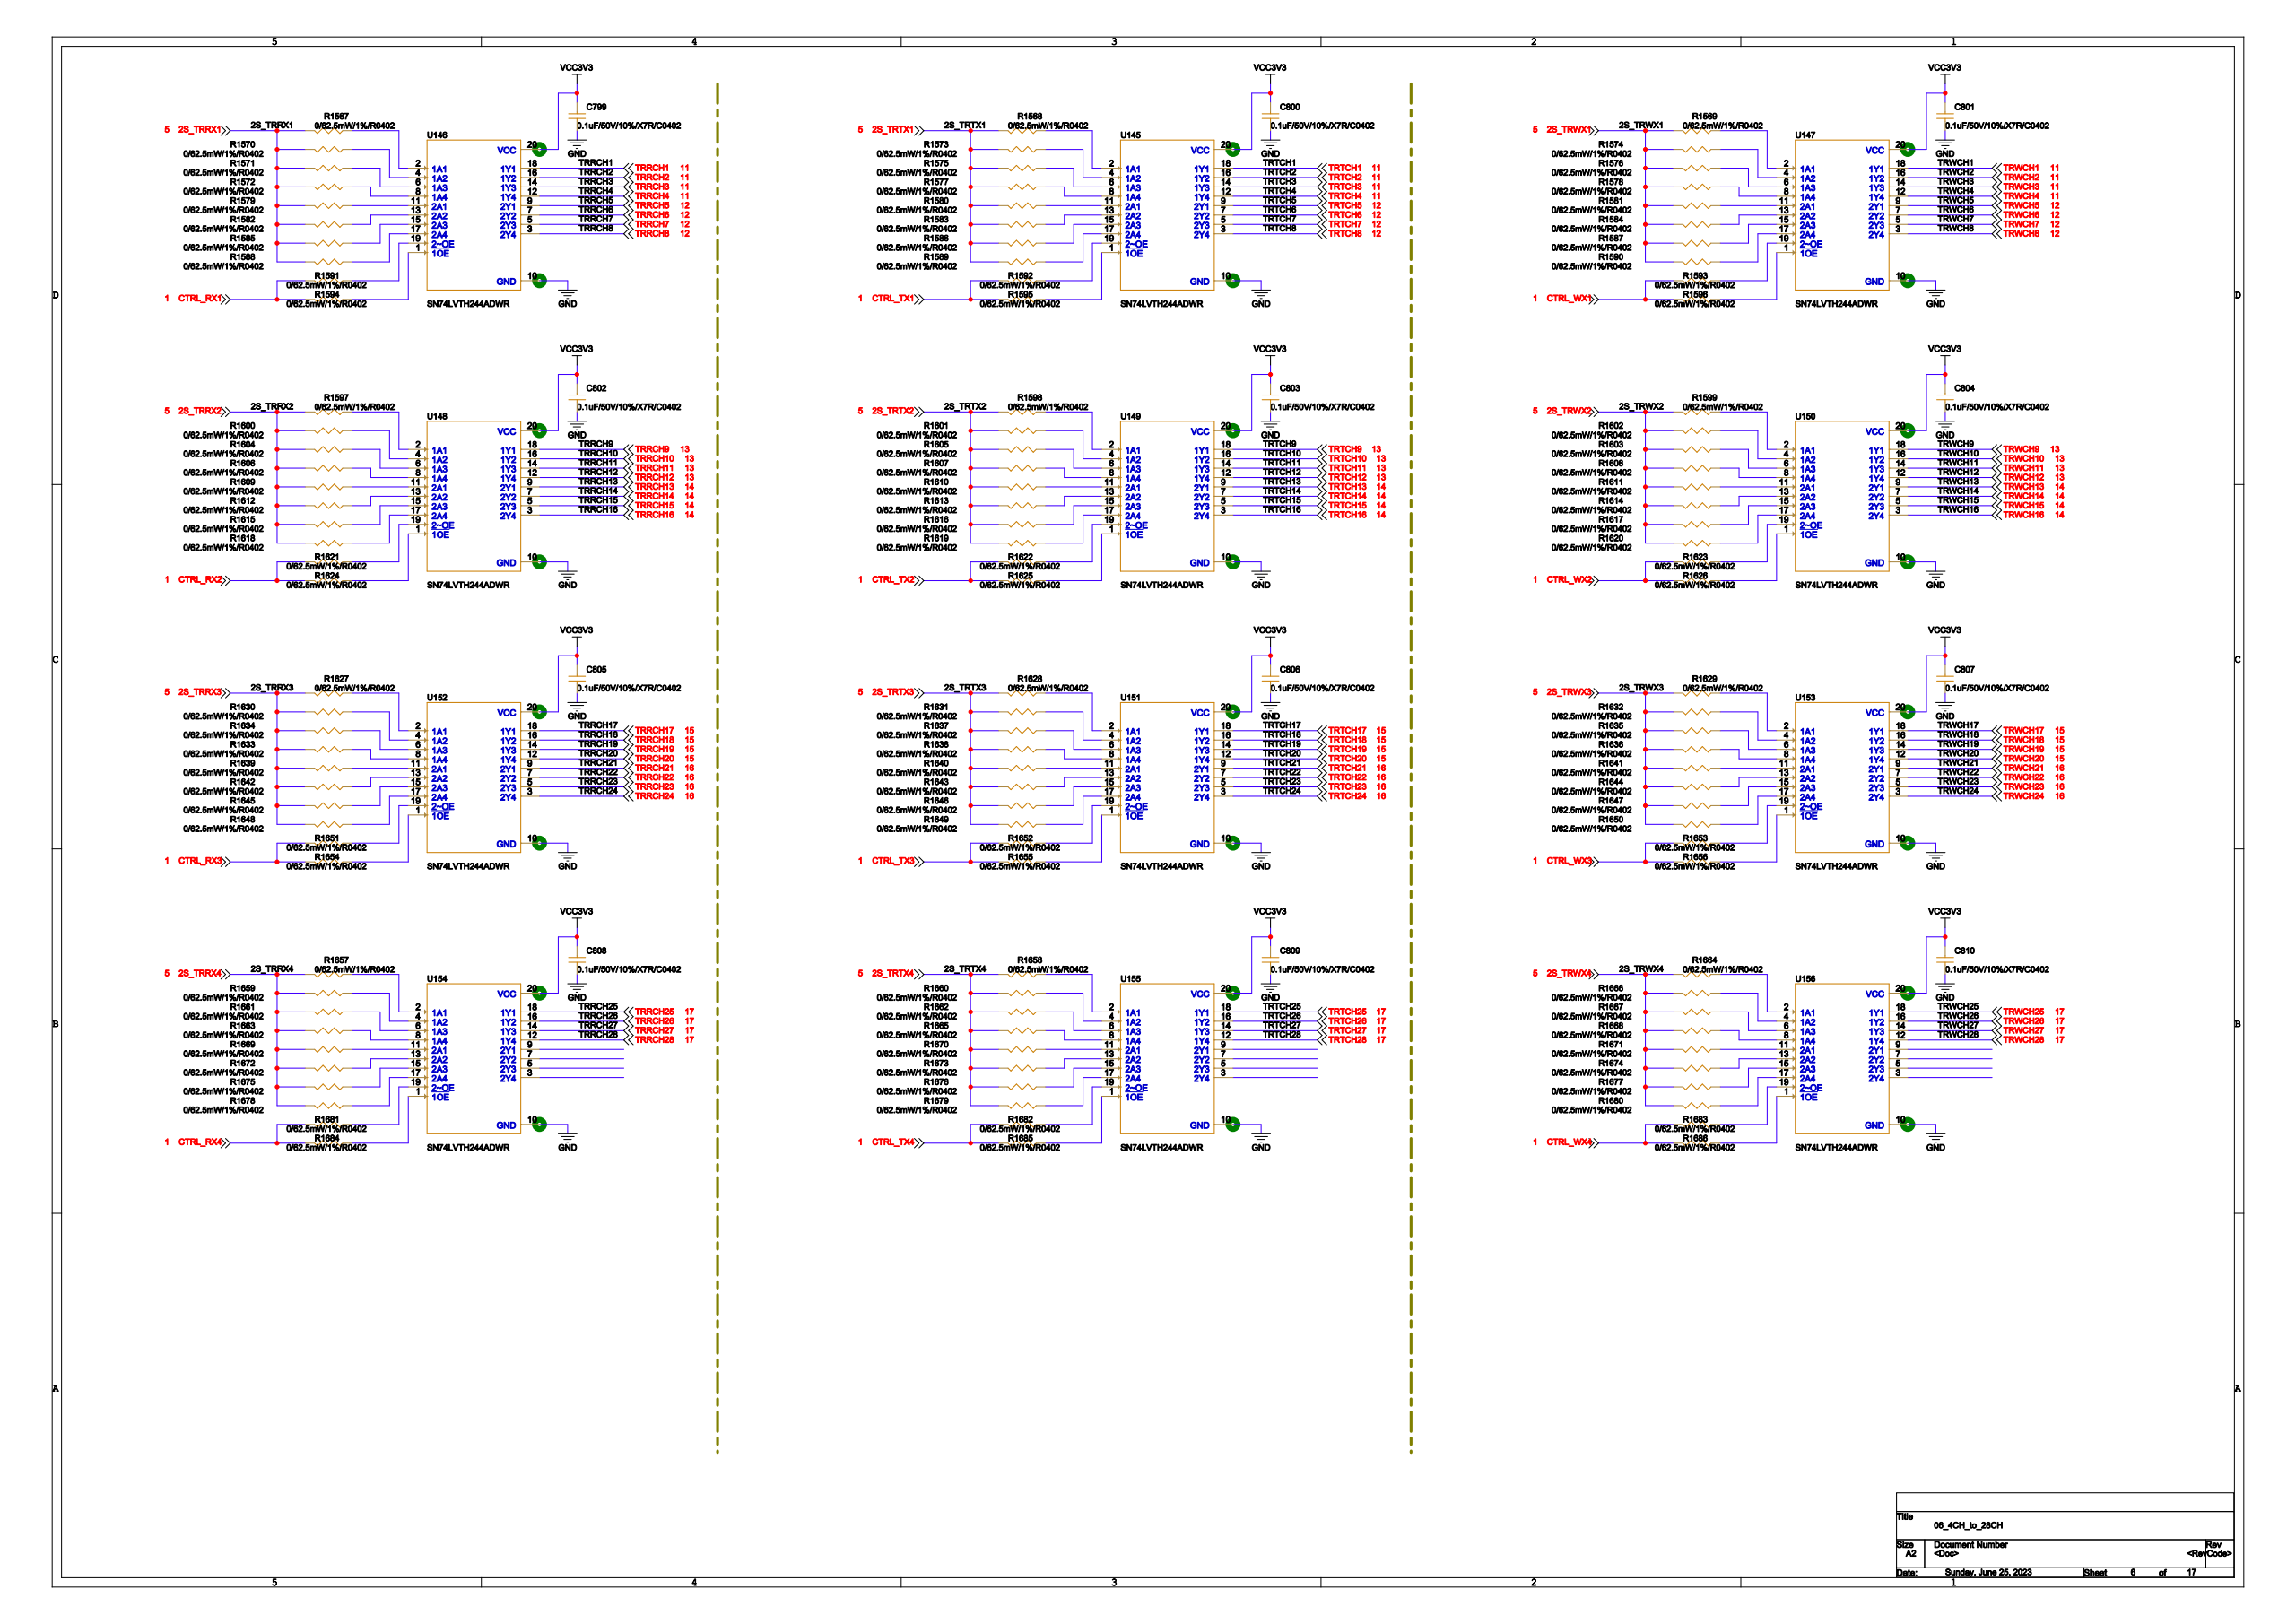Circuit board | Cadence Allegro | 2002 parts | 1538 nets | one sheet of the schematic
Parts on this sheet (reference | value | footprint):
C799 | 0.1uF/50V/10%/X7R/C0402 | 0402
C800 | 0.1uF/50V/10%/X7R/C0402 | 0402
C801 | 0.1uF/50V/10%/X7R/C0402 | 0402
C802 | 0.1uF/50V/10%/X7R/C0402 | 0402
C803 | 0.1uF/50V/10%/X7R/C0402 | 0402
C804 | 0.1uF/50V/10%/X7R/C0402 | 0402
C805 | 0.1uF/50V/10%/X7R/C0402 | 0402
C806 | 0.1uF/50V/10%/X7R/C0402 | 0402
C807 | 0.1uF/50V/10%/X7R/C0402 | 0402
C808 | 0.1uF/50V/10%/X7R/C0402 | 0402
C809 | 0.1uF/50V/10%/X7R/C0402 | 0402
C810 | 0.1uF/50V/10%/X7R/C0402 | 0402
R1567 | 0/62.5mW/1%/R0402 | 0402
R1568 | 0/62.5mW/1%/R0402 | 0402
R1569 | 0/62.5mW/1%/R0402 | 0402
R1570 | 0/62.5mW/1%/R0402 | 0402
R1571 | 0/62.5mW/1%/R0402 | 0402
R1572 | 0/62.5mW/1%/R0402 | 0402
R1573 | 0/62.5mW/1%/R0402 | 0402
R1574 | 0/62.5mW/1%/R0402 | 0402
R1575 | 0/62.5mW/1%/R0402 | 0402
R1576 | 0/62.5mW/1%/R0402 | 0402
R1577 | 0/62.5mW/1%/R0402 | 0402
R1578 | 0/62.5mW/1%/R0402 | 0402
R1579 | 0/62.5mW/1%/R0402 | 0402
R1580 | 0/62.5mW/1%/R0402 | 0402
R1581 | 0/62.5mW/1%/R0402 | 0402
R1582 | 0/62.5mW/1%/R0402 | 0402
R1583 | 0/62.5mW/1%/R0402 | 0402
R1584 | 0/62.5mW/1%/R0402 | 0402
R1585 | 0/62.5mW/1%/R0402 | 0402
R1586 | 0/62.5mW/1%/R0402 | 0402
R1587 | 0/62.5mW/1%/R0402 | 0402
R1588 | 0/62.5mW/1%/R0402 | 0402
R1589 | 0/62.5mW/1%/R0402 | 0402
R1590 | 0/62.5mW/1%/R0402 | 0402
R1591 | 0/62.5mW/1%/R0402 | 0402
R1592 | 0/62.5mW/1%/R0402 | 0402
R1593 | 0/62.5mW/1%/R0402 | 0402
R1594 | 0/62.5mW/1%/R0402 | 0402
R1595 | 0/62.5mW/1%/R0402 | 0402
R1596 | 0/62.5mW/1%/R0402 | 0402
R1597 | 0/62.5mW/1%/R0402 | 0402
R1598 | 0/62.5mW/1%/R0402 | 0402
R1599 | 0/62.5mW/1%/R0402 | 0402
R1600 | 0/62.5mW/1%/R0402 | 0402
R1601 | 0/62.5mW/1%/R0402 | 0402
R1602 | 0/62.5mW/1%/R0402 | 0402
R1603 | 0/62.5mW/1%/R0402 | 0402
R1604 | 0/62.5mW/1%/R0402 | 0402
R1605 | 0/62.5mW/1%/R0402 | 0402
R1606 | 0/62.5mW/1%/R0402 | 0402
R1607 | 0/62.5mW/1%/R0402 | 0402
R1608 | 0/62.5mW/1%/R0402 | 0402
R1609 | 0/62.5mW/1%/R0402 | 0402
R1610 | 0/62.5mW/1%/R0402 | 0402
R1611 | 0/62.5mW/1%/R0402 | 0402
R1612 | 0/62.5mW/1%/R0402 | 0402
R1613 | 0/62.5mW/1%/R0402 | 0402
R1614 | 0/62.5mW/1%/R0402 | 0402
R1615 | 0/62.5mW/1%/R0402 | 0402
R1616 | 0/62.5mW/1%/R0402 | 0402
R1617 | 0/62.5mW/1%/R0402 | 0402
R1618 | 0/62.5mW/1%/R0402 | 0402
R1619 | 0/62.5mW/1%/R0402 | 0402
R1620 | 0/62.5mW/1%/R0402 | 0402
R1621 | 0/62.5mW/1%/R0402 | 0402
R1622 | 0/62.5mW/1%/R0402 | 0402
R1623 | 0/62.5mW/1%/R0402 | 0402
R1624 | 0/62.5mW/1%/R0402 | 0402
R1625 | 0/62.5mW/1%/R0402 | 0402
R1626 | 0/62.5mW/1%/R0402 | 0402
R1627 | 0/62.5mW/1%/R0402 | 0402
R1628 | 0/62.5mW/1%/R0402 | 0402
R1629 | 0/62.5mW/1%/R0402 | 0402
R1630 | 0/62.5mW/1%/R0402 | 0402
R1631 | 0/62.5mW/1%/R0402 | 0402
R1632 | 0/62.5mW/1%/R0402 | 0402
R1633 | 0/62.5mW/1%/R0402 | 0402
R1634 | 0/62.5mW/1%/R0402 | 0402
R1635 | 0/62.5mW/1%/R0402 | 0402
R1636 | 0/62.5mW/1%/R0402 | 0402
R1637 | 0/62.5mW/1%/R0402 | 0402
R1638 | 0/62.5mW/1%/R0402 | 0402
R1639 | 0/62.5mW/1%/R0402 | 0402
R1640 | 0/62.5mW/1%/R0402 | 0402
R1641 | 0/62.5mW/1%/R0402 | 0402
R1642 | 0/62.5mW/1%/R0402 | 0402
R1643 | 0/62.5mW/1%/R0402 | 0402
R1644 | 0/62.5mW/1%/R0402 | 0402
R1645 | 0/62.5mW/1%/R0402 | 0402
R1646 | 0/62.5mW/1%/R0402 | 0402
R1647 | 0/62.5mW/1%/R0402 | 0402
R1648 | 0/62.5mW/1%/R0402 | 0402
R1649 | 0/62.5mW/1%/R0402 | 0402
R1650 | 0/62.5mW/1%/R0402 | 0402
R1651 | 0/62.5mW/1%/R0402 | 0402
R1652 | 0/62.5mW/1%/R0402 | 0402
R1653 | 0/62.5mW/1%/R0402 | 0402
R1654 | 0/62.5mW/1%/R0402 | 0402
R1655 | 0/62.5mW/1%/R0402 | 0402
R1656 | 0/62.5mW/1%/R0402 | 0402
R1657 | 0/62.5mW/1%/R0402 | 0402
R1658 | 0/62.5mW/1%/R0402 | 0402
R1659 | 0/62.5mW/1%/R0402 | 0402
R1660 | 0/62.5mW/1%/R0402 | 0402
R1661 | 0/62.5mW/1%/R0402 | 0402
R1662 | 0/62.5mW/1%/R0402 | 0402
R1663 | 0/62.5mW/1%/R0402 | 0402
R1664 | 0/62.5mW/1%/R0402 | 0402
R1665 | 0/62.5mW/1%/R0402 | 0402
R1666 | 0/62.5mW/1%/R0402 | 0402
R1667 | 0/62.5mW/1%/R0402 | 0402
R1668 | 0/62.5mW/1%/R0402 | 0402
R1669 | 0/62.5mW/1%/R0402 | 0402
R1670 | 0/62.5mW/1%/R0402 | 0402
R1671 | 0/62.5mW/1%/R0402 | 0402
R1672 | 0/62.5mW/1%/R0402 | 0402
R1673 | 0/62.5mW/1%/R0402 | 0402
R1674 | 0/62.5mW/1%/R0402 | 0402
R1675 | 0/62.5mW/1%/R0402 | 0402
R1676 | 0/62.5mW/1%/R0402 | 0402
R1677 | 0/62.5mW/1%/R0402 | 0402
R1678 | 0/62.5mW/1%/R0402 | 0402
R1679 | 0/62.5mW/1%/R0402 | 0402
R1680 | 0/62.5mW/1%/R0402 | 0402
R1681 | 0/62.5mW/1%/R0402 | 0402
R1682 | 0/62.5mW/1%/R0402 | 0402
R1683 | 0/62.5mW/1%/R0402 | 0402
R1684 | 0/62.5mW/1%/R0402 | 0402
R1685 | 0/62.5mW/1%/R0402 | 0402
R1686 | 0/62.5mW/1%/R0402 | 0402
U145 | SN74LVTH244ADWR | SOIC127P1030X265-20N
U146 | SN74LVTH244ADWR | SOIC127P1030X265-20N
U147 | SN74LVTH244ADWR | SOIC127P1030X265-20N
U148 | SN74LVTH244ADWR | SOIC127P1030X265-20N
U149 | SN74LVTH244ADWR | SOIC127P1030X265-20N
U150 | SN74LVTH244ADWR | SOIC127P1030X265-20N
U151 | SN74LVTH244ADWR | SOIC127P1030X265-20N
U152 | SN74LVTH244ADWR | SOIC127P1030X265-20N
U153 | SN74LVTH244ADWR | SOIC127P1030X265-20N
U154 | SN74LVTH244ADWR | SOIC127P1030X265-20N
U155 | SN74LVTH244ADWR | SOIC127P1030X265-20N
U156 | SN74LVTH244ADWR | SOIC127P1030X265-20N
Nets of these parts (net: part-pin ...):
3.3V: C799-1 C800-1 C801-1 C802-1 C803-1 C804-1 C805-1 C806-1 C807-1 C808-1 C809-1 C810-1 U145-20 U146-20 U147-20 U148-20 U149-20 U150-20 U151-20 U152-20 U153-20 U154-20 U155-20 U156-20
AGND: C799-2 C800-2 C801-2 C802-2 C803-2 C804-2 C805-2 C806-2 C807-2 C808-2 C809-2 C810-2 U145-10 U146-10 U147-10 U148-10 U149-10 U150-10 U151-10 U152-10 U153-10 U154-10 U155-10 U156-10
CTRL_RX3: R1651-1 R1654-1
CTRL_RX2: R1621-1 R1624-1
CTRL_WX2: R1623-1 R1626-1
CTRL_TX2: R1622-1 R1625-1
CTRL_TX1: R1592-1 R1595-1
CTRL_WX4: R1683-1 R1686-1
CTRL_RX1: R1591-1 R1594-1
CTRL_WX1: R1593-1 R1596-1
CTRL_RX4: R1681-1 R1684-1
CTRL_TX4: R1682-1 R1685-1
CTRL_WX3: R1653-1 R1656-1
CTRL_TX3: R1652-1 R1655-1
2S_TRRX1: R1567-1 R1570-1 R1571-1 R1572-1 R1579-1 R1582-1 R1585-1 R1588-1
N23955636: R1567-2 U146-2
2S_TRTX1: R1568-1 R1573-1 R1575-1 R1577-1 R1580-1 R1583-1 R1586-1 R1589-1
N23963258: R1568-2 U145-2
2S_TRWX1: R1569-1 R1574-1 R1576-1 R1578-1 R1581-1 R1584-1 R1587-1 R1590-1
N23976669: R1569-2 U147-2
N23955843: R1570-2 U146-4
N23955864: R1571-2 U146-6
N23955873: R1572-2 U146-8
N23963345: R1573-2 U145-4
N23976782: R1574-2 U147-4
N23963355: R1575-2 U145-6
N23976792: R1576-2 U147-6
N23963361: R1577-2 U145-8
N23976798: R1578-2 U147-8
N23955883: R1579-2 U146-11
N23963367: R1580-2 U145-11
N23976804: R1581-2 U147-11
N23955886: R1582-2 U146-13
N23963369: R1583-2 U145-13
N23976806: R1584-2 U147-13
N23955895: R1585-2 U146-15
N23963375: R1586-2 U145-15
N23976812: R1587-2 U147-15
N23955904: R1588-2 U146-17
N23963381: R1589-2 U145-17
N23976818: R1590-2 U147-17
N23955981: R1591-2 U146-19
N23963403: R1592-2 U145-19
N23976840: R1593-2 U147-19
N23955993: R1594-2 U146-1
N23963409: R1595-2 U145-1
N23976846: R1596-2 U147-1
2S_TRRX2: R1597-1 R1600-1 R1604-1 R1606-1 R1609-1 R1612-1 R1615-1 R1618-1
N23957290: R1597-2 U148-2
2S_TRTX2: R1598-1 R1601-1 R1605-1 R1607-1 R1610-1 R1613-1 R1616-1 R1619-1
N23963537: R1598-2 U149-2
2S_TRWX2: R1599-1 R1602-1 R1603-1 R1608-1 R1611-1 R1614-1 R1617-1 R1620-1
N23976942: R1599-2 U150-2
N23957377: R1600-2 U148-4
N23963650: R1601-2 U149-4
N23977055: R1602-2 U150-4
N23977065: R1603-2 U150-6
N23957387: R1604-2 U148-6
N23963660: R1605-2 U149-6
N23957393: R1606-2 U148-8
N23963666: R1607-2 U149-8
N23977071: R1608-2 U150-8
N23957399: R1609-2 U148-11
N23963672: R1610-2 U149-11
N23977077: R1611-2 U150-11
N23957401: R1612-2 U148-13
N23963674: R1613-2 U149-13
N23977079: R1614-2 U150-13
N23957407: R1615-2 U148-15
N23963680: R1616-2 U149-15
N23977085: R1617-2 U150-15
N23957413: R1618-2 U148-17
N23963686: R1619-2 U149-17
N23977091: R1620-2 U150-17
N23957435: R1621-2 U148-19
N23963708: R1622-2 U149-19
N23977113: R1623-2 U150-19
N23957441: R1624-2 U148-1
N23963714: R1625-2 U149-1
N23977119: R1626-2 U150-1
2S_TRRX3: R1627-1 R1630-1 R1633-1 R1634-1 R1639-1 R1642-1 R1645-1 R1648-1
N23958041: R1627-2 U152-2
2S_TRTX3: R1628-1 R1631-1 R1637-1 R1638-1 R1640-1 R1643-1 R1646-1 R1649-1
N23963810: R1628-2 U151-2
2S_TRWX3: R1629-1 R1632-1 R1635-1 R1636-1 R1641-1 R1644-1 R1647-1 R1650-1
N23977215: R1629-2 U153-2
N23958128: R1630-2 U152-4
N23963923: R1631-2 U151-4
N23977328: R1632-2 U153-4
N23958144: R1633-2 U152-8
N23958138: R1634-2 U152-6
N23977338: R1635-2 U153-6
N23977344: R1636-2 U153-8
N23963933: R1637-2 U151-6
N23963939: R1638-2 U151-8
N23958150: R1639-2 U152-11
N23963945: R1640-2 U151-11
N23977350: R1641-2 U153-11
N23958152: R1642-2 U152-13
N23963947: R1643-2 U151-13
N23977352: R1644-2 U153-13
N23958158: R1645-2 U152-15
N23963953: R1646-2 U151-15
N23977358: R1647-2 U153-15
N23958164: R1648-2 U152-17
N23963959: R1649-2 U151-17
N23977364: R1650-2 U153-17
N23958186: R1651-2 U152-19
N23963981: R1652-2 U151-19
N23977386: R1653-2 U153-19
N23958192: R1654-2 U152-1
N23963987: R1655-2 U151-1
N23977392: R1656-2 U153-1
2S_TRRX4: R1657-1 R1659-1 R1661-1 R1663-1 R1669-1 R1672-1 R1675-1 R1678-1
N23958837: R1657-2 U154-2
2S_TRTX4: R1658-1 R1660-1 R1662-1 R1665-1 R1670-1 R1673-1 R1676-1 R1679-1
N23964083: R1658-2 U155-2
N23958924: R1659-2 U154-4
N23964196: R1660-2 U155-4
N23958934: R1661-2 U154-6
N23964206: R1662-2 U155-6
N23958940: R1663-2 U154-8
2S_TRWX4: R1664-1 R1666-1 R1667-1 R1668-1 R1671-1 R1674-1 R1677-1 R1680-1
N23977488: R1664-2 U156-2
N23964212: R1665-2 U155-8
N23977601: R1666-2 U156-4
N23977611: R1667-2 U156-6
N23977617: R1668-2 U156-8
N23958946: R1669-2 U154-11
N23964218: R1670-2 U155-11
N23977623: R1671-2 U156-11
N23958948: R1672-2 U154-13
N23964220: R1673-2 U155-13
N23977625: R1674-2 U156-13
N23958954: R1675-2 U154-15
N23964226: R1676-2 U155-15
N23977631: R1677-2 U156-15
N23958960: R1678-2 U154-17
N23964232: R1679-2 U155-17
N23977637: R1680-2 U156-17
N23958982: R1681-2 U154-19
N23964254: R1682-2 U155-19
N23977659: R1683-2 U156-19
N23958988: R1684-2 U154-1
N23964260: R1685-2 U155-1
N23977665: R1686-2 U156-1
TRRCH1: U146-18
TRTCH1: U145-18
TRWCH1: U147-18
TRRCH2: U146-16
TRTCH2: U145-16
TRWCH2: U147-16
TRRCH3: U146-14
TRTCH3: U145-14
TRWCH3: U147-14
TRRCH4: U146-12
TRTCH4: U145-12
TRWCH4: U147-12
TRRCH5: U146-9
TRTCH5: U145-9
TRWCH5: U147-9
TRRCH6: U146-7
TRTCH6: U145-7
TRWCH6: U147-7
TRTCH7: U145-5
TRRCH7: U146-5
TRWCH7: U147-5
TRRCH8: U146-3
TRTCH8: U145-3
TRWCH8: U147-3
TRRCH9: U148-18
TRTCH9: U149-18
TRWCH9: U150-18
TRRCH10: U148-16
TRTCH10: U149-16
TRWCH10: U150-16
TRRCH11: U148-14
TRTCH11: U149-14
TRWCH11: U150-14
TRRCH12: U148-12
TRTCH12: U149-12
TRWCH12: U150-12
TRRCH13: U148-9
TRTCH13: U149-9
TRWCH13: U150-9
TRTCH14: U149-7
TRRCH14: U148-7
TRWCH14: U150-7
TRTCH15: U149-5
TRWCH15: U150-5
TRRCH15: U148-5
TRRCH16: U148-3
TRTCH16: U149-3
TRWCH16: U150-3
TRRCH17: U152-18
TRTCH17: U151-18
TRWCH17: U153-18
TRRCH18: U152-16
TRTCH18: U151-16
TRWCH18: U153-16
TRRCH19: U152-14
TRTCH19: U151-14
TRWCH19: U153-14
TRRCH20: U152-12
TRTCH20: U151-12
TRWCH20: U153-12
TRRCH21: U152-9
TRTCH21: U151-9
TRWCH21: U153-9
TRRCH22: U152-7
TRTCH22: U151-7
TRWCH22: U153-7
TRRCH23: U152-5
TRTCH23: U151-5
TRWCH23: U153-5
TRRCH24: U152-3
TRTCH24: U151-3
TRWCH24: U153-3
TRRCH25: U154-18
TRTCH25: U155-18
TRWCH25: U156-18
TRRCH26: U154-16
TRTCH26: U155-16
TRWCH26: U156-16
TRRCH27: U154-14
TRTCH27: U155-14
TRWCH27: U156-14
TRRCH28: U154-12
TRWCH28: U156-12
TRTCH28: U155-12
N23959088: U154-9
N23959091: U154-7
N23959102: U154-5
N23959105: U154-3
N23964344: U155-9
N23964347: U155-7
N23964350: U155-5
N23964353: U155-3
N23977749: U156-9
N23977752: U156-7
N23977755: U156-5
N23977758: U156-3